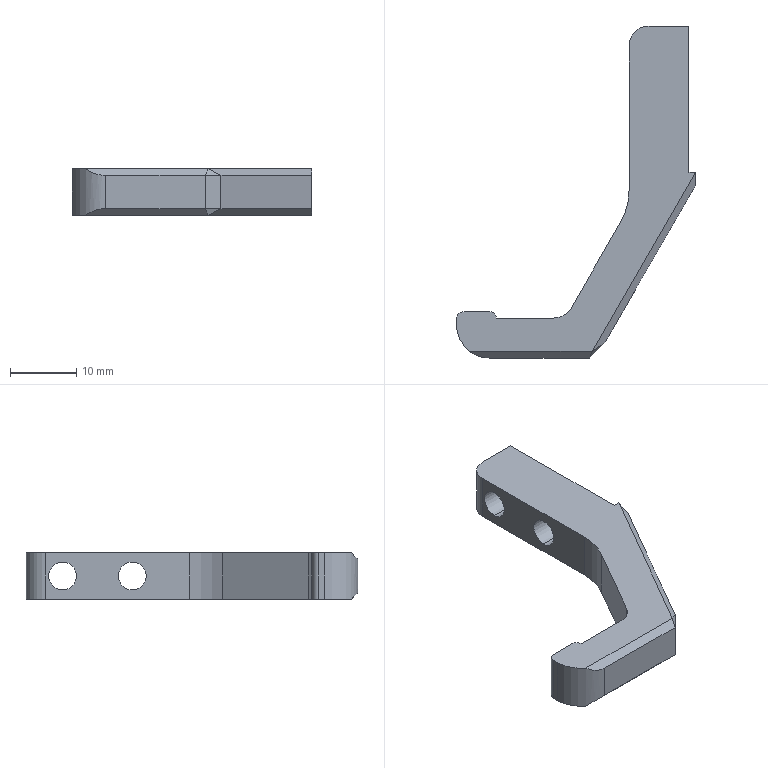Part | NX | features BREP 1 | 1 solid | 30 faces | box 36 x 49.981 x 7 mm | volume 3323 mm3 | plane 20 | cylinder 10 | commonest cylinder face diameters 4.2 x4 2 x2 6 x2 10 x1 20 x1
STEP:
#1=CARTESIAN_POINT('',(733.282,0.5081,5.6));
#2=VERTEX_POINT('',#1);
#3=CARTESIAN_POINT('',(733.282,0.5081,1.4));
#4=VERTEX_POINT('',#3);
#5=CARTESIAN_POINT('',(733.282,0.5081,3.5));
#6=DIRECTION('',(1.,0.,0.));
#7=DIRECTION('',(0.,1.,0.));
#8=AXIS2_PLACEMENT_3D('',#5,#6,#7);
#9=CIRCLE('',#8,2.1);
#10=EDGE_CURVE('',#2,#4,#9,.T.);
#11=ORIENTED_EDGE('',*,*,#10,.F.);
#12=CARTESIAN_POINT('',(742.282,0.5081,5.6));
#13=VERTEX_POINT('',#12);
#14=CARTESIAN_POINT('',(742.282,0.5081,5.6));
#15=DIRECTION('',(1.,0.,0.));
#16=VECTOR('',#15,1000.);
#17=LINE('',#14,#16);
#18=EDGE_CURVE('',#2,#13,#17,.T.);
#19=ORIENTED_EDGE('',*,*,#18,.T.);
#20=CARTESIAN_POINT('',(742.282,0.5081,1.4));
#21=VERTEX_POINT('',#20);
#22=CARTESIAN_POINT('',(742.282,0.5081,3.5));
#23=DIRECTION('',(1.,0.,0.));
#24=DIRECTION('',(0.,0.,-1.));
#25=AXIS2_PLACEMENT_3D('',#22,#23,#24);
#26=CIRCLE('',#25,2.1);
#27=EDGE_CURVE('',#13,#21,#26,.T.);
#28=ORIENTED_EDGE('',*,*,#27,.T.);
#29=CARTESIAN_POINT('',(742.282,0.5081,1.4));
#30=DIRECTION('',(1.,0.,0.));
#31=VECTOR('',#30,1000.);
#32=LINE('',#29,#31);
#33=EDGE_CURVE('',#4,#21,#32,.T.);
#34=ORIENTED_EDGE('',*,*,#33,.F.);
#35=EDGE_LOOP('',(#11,#19,#28,#34));
#36=FACE_BOUND('',#35,.T.);
#37=CARTESIAN_POINT('',(742.282,0.5081,3.5));
#38=DIRECTION('',(1.,0.,0.));
#39=DIRECTION('',(0.,0.,-1.));
#40=AXIS2_PLACEMENT_3D('',#37,#38,#39);
#41=CYLINDRICAL_SURFACE('',#40,2.1);
#42=ADVANCED_FACE('',(#36),#41,.F.);
#43=CARTESIAN_POINT('',(733.282,11.008,5.6));
#44=VERTEX_POINT('',#43);
#45=CARTESIAN_POINT('',(733.282,11.008,1.4));
#46=VERTEX_POINT('',#45);
#47=CARTESIAN_POINT('',(733.282,11.008,3.5));
#48=DIRECTION('',(1.,0.,0.));
#49=DIRECTION('',(0.,1.,0.));
#50=AXIS2_PLACEMENT_3D('',#47,#48,#49);
#51=CIRCLE('',#50,2.1);
#52=EDGE_CURVE('',#44,#46,#51,.T.);
#53=ORIENTED_EDGE('',*,*,#52,.F.);
#54=CARTESIAN_POINT('',(742.282,11.008,5.6));
#55=VERTEX_POINT('',#54);
#56=CARTESIAN_POINT('',(742.282,11.008,5.6));
#57=DIRECTION('',(1.,0.,0.));
#58=VECTOR('',#57,1000.);
#59=LINE('',#56,#58);
#60=EDGE_CURVE('',#44,#55,#59,.T.);
#61=ORIENTED_EDGE('',*,*,#60,.T.);
#62=CARTESIAN_POINT('',(742.282,11.008,1.4));
#63=VERTEX_POINT('',#62);
#64=CARTESIAN_POINT('',(742.282,11.008,3.5));
#65=DIRECTION('',(1.,0.,0.));
#66=DIRECTION('',(0.,0.,-1.));
#67=AXIS2_PLACEMENT_3D('',#64,#65,#66);
#68=CIRCLE('',#67,2.1);
#69=EDGE_CURVE('',#55,#63,#68,.T.);
#70=ORIENTED_EDGE('',*,*,#69,.T.);
#71=CARTESIAN_POINT('',(742.282,11.008,1.4));
#72=DIRECTION('',(1.,0.,0.));
#73=VECTOR('',#72,1000.);
#74=LINE('',#71,#73);
#75=EDGE_CURVE('',#46,#63,#74,.T.);
#76=ORIENTED_EDGE('',*,*,#75,.F.);
#77=EDGE_LOOP('',(#53,#61,#70,#76));
#78=FACE_BOUND('',#77,.T.);
#79=CARTESIAN_POINT('',(742.282,11.008,3.5));
#80=DIRECTION('',(1.,0.,0.));
#81=DIRECTION('',(0.,0.,-1.));
#82=AXIS2_PLACEMENT_3D('',#79,#80,#81);
#83=CYLINDRICAL_SURFACE('',#82,2.1);
#84=ADVANCED_FACE('',(#78),#83,.F.);
#85=CARTESIAN_POINT('',(707.282,-27.556,7.));
#86=VERTEX_POINT('',#85);
#87=CARTESIAN_POINT('',(707.282,-28.473,7.));
#88=VERTEX_POINT('',#87);
#89=CARTESIAN_POINT('',(707.282,-26.473,7.));
#90=DIRECTION('',(0.,-1.,0.));
#91=VECTOR('',#90,1000.);
#92=LINE('',#89,#91);
#93=EDGE_CURVE('',#86,#88,#92,.T.);
#94=ORIENTED_EDGE('',*,*,#93,.F.);
#95=CARTESIAN_POINT('',(707.282,-27.556,0.));
#96=VERTEX_POINT('',#95);
#97=CARTESIAN_POINT('',(707.282,-27.556,0.));
#98=DIRECTION('',(0.,0.,-1.));
#99=VECTOR('',#98,1000.);
#100=LINE('',#97,#99);
#101=EDGE_CURVE('',#86,#96,#100,.T.);
#102=ORIENTED_EDGE('',*,*,#101,.T.);
#103=CARTESIAN_POINT('',(707.282,-28.473,0.));
#104=VERTEX_POINT('',#103);
#105=CARTESIAN_POINT('',(707.282,-26.473,0.));
#106=DIRECTION('',(0.,-1.,0.));
#107=VECTOR('',#106,1000.);
#108=LINE('',#105,#107);
#109=EDGE_CURVE('',#96,#104,#108,.T.);
#110=ORIENTED_EDGE('',*,*,#109,.T.);
#111=CARTESIAN_POINT('',(707.282,-28.473,7.));
#112=DIRECTION('',(0.,0.,1.));
#113=VECTOR('',#112,1000.);
#114=LINE('',#111,#113);
#115=EDGE_CURVE('',#104,#88,#114,.T.);
#116=ORIENTED_EDGE('',*,*,#115,.T.);
#117=EDGE_LOOP('',(#94,#102,#110,#116));
#118=FACE_BOUND('',#117,.T.);
#119=CARTESIAN_POINT('',(707.282,-26.473,7.));
#120=DIRECTION('',(1.,0.,0.));
#121=DIRECTION('',(0.,1.,0.));
#122=AXIS2_PLACEMENT_3D('',#119,#120,#121);
#123=PLANE('',#122);
#124=ADVANCED_FACE('',(#118),#123,.F.);
#125=CARTESIAN_POINT('',(712.265,-26.49,7.));
#126=VERTEX_POINT('',#125);
#127=CARTESIAN_POINT('',(708.265,-26.556,7.));
#128=VERTEX_POINT('',#127);
#129=CARTESIAN_POINT('',(707.167,-26.575,7.));
#130=DIRECTION('',(-0.9999,-0.01666,0.));
#131=VECTOR('',#130,1000.);
#132=LINE('',#129,#131);
#133=EDGE_CURVE('',#126,#128,#132,.T.);
#134=ORIENTED_EDGE('',*,*,#133,.T.);
#135=CARTESIAN_POINT('',(708.282,-27.556,7.));
#136=DIRECTION('',(0.,0.,1.));
#137=DIRECTION('',(1.,0.,0.));
#138=AXIS2_PLACEMENT_3D('',#135,#136,#137);
#139=CIRCLE('',#138,1.);
#140=EDGE_CURVE('',#128,#86,#139,.T.);
#141=ORIENTED_EDGE('',*,*,#140,.T.);
#142=ORIENTED_EDGE('',*,*,#93,.T.);
#143=CARTESIAN_POINT('',(709.282,-32.473,7.));
#144=VERTEX_POINT('',#143);
#145=CARTESIAN_POINT('',(712.282,-28.473,7.));
#146=DIRECTION('',(0.,0.,1.));
#147=DIRECTION('',(1.,0.,0.));
#148=AXIS2_PLACEMENT_3D('',#145,#146,#147);
#149=CIRCLE('',#148,5.);
#150=EDGE_CURVE('',#88,#144,#149,.T.);
#151=ORIENTED_EDGE('',*,*,#150,.T.);
#152=CARTESIAN_POINT('',(727.704,-32.473,7.));
#153=VERTEX_POINT('',#152);
#154=CARTESIAN_POINT('',(728.282,-32.473,7.));
#155=DIRECTION('',(1.,0.,0.));
#156=VECTOR('',#155,1000.);
#157=LINE('',#154,#156);
#158=EDGE_CURVE('',#144,#153,#157,.T.);
#159=ORIENTED_EDGE('',*,*,#158,.T.);
#160=CARTESIAN_POINT('',(743.282,-5.492,7.));
#161=VERTEX_POINT('',#160);
#162=CARTESIAN_POINT('',(742.416,-6.992,7.));
#163=DIRECTION('',(0.5,0.866,0.));
#164=VECTOR('',#163,1000.);
#165=LINE('',#162,#164);
#166=EDGE_CURVE('',#153,#161,#165,.T.);
#167=ORIENTED_EDGE('',*,*,#166,.T.);
#168=CARTESIAN_POINT('',(742.282,-5.492,7.));
#169=VERTEX_POINT('',#168);
#170=CARTESIAN_POINT('',(743.282,-5.492,7.));
#171=DIRECTION('',(1.,0.,0.));
#172=VECTOR('',#171,1000.);
#173=LINE('',#170,#172);
#174=EDGE_CURVE('',#169,#161,#173,.T.);
#175=ORIENTED_EDGE('',*,*,#174,.F.);
#176=CARTESIAN_POINT('',(742.282,16.508,7.));
#177=VERTEX_POINT('',#176);
#178=CARTESIAN_POINT('',(742.282,-5.492,7.));
#179=DIRECTION('',(0.,-1.,0.));
#180=VECTOR('',#179,1000.);
#181=LINE('',#178,#180);
#182=EDGE_CURVE('',#177,#169,#181,.T.);
#183=ORIENTED_EDGE('',*,*,#182,.F.);
#184=CARTESIAN_POINT('',(736.282,16.508,7.));
#185=VERTEX_POINT('',#184);
#186=CARTESIAN_POINT('',(743.282,16.508,7.));
#187=DIRECTION('',(-1.,0.,0.));
#188=VECTOR('',#187,1000.);
#189=LINE('',#186,#188);
#190=EDGE_CURVE('',#177,#185,#189,.T.);
#191=ORIENTED_EDGE('',*,*,#190,.T.);
#192=CARTESIAN_POINT('',(733.282,13.508,7.));
#193=VERTEX_POINT('',#192);
#194=CARTESIAN_POINT('',(736.282,13.508,7.));
#195=DIRECTION('',(0.,0.,1.));
#196=DIRECTION('',(1.,0.,0.));
#197=AXIS2_PLACEMENT_3D('',#194,#195,#196);
#198=CIRCLE('',#197,3.);
#199=EDGE_CURVE('',#185,#193,#198,.T.);
#200=ORIENTED_EDGE('',*,*,#199,.T.);
#201=CARTESIAN_POINT('',(733.282,-8.133,7.));
#202=VERTEX_POINT('',#201);
#203=CARTESIAN_POINT('',(733.282,-10.812,7.));
#204=DIRECTION('',(0.,-1.,0.));
#205=VECTOR('',#204,1000.);
#206=LINE('',#203,#205);
#207=EDGE_CURVE('',#193,#202,#206,.T.);
#208=ORIENTED_EDGE('',*,*,#207,.T.);
#209=CARTESIAN_POINT('',(731.942,-13.133,7.));
#210=VERTEX_POINT('',#209);
#211=CARTESIAN_POINT('',(723.282,-8.133,7.));
#212=DIRECTION('',(0.,0.,-1.));
#213=DIRECTION('',(1.,0.,0.));
#214=AXIS2_PLACEMENT_3D('',#211,#212,#213);
#215=CIRCLE('',#214,10.);
#216=EDGE_CURVE('',#202,#210,#215,.T.);
#217=ORIENTED_EDGE('',*,*,#216,.T.);
#218=CARTESIAN_POINT('',(724.529,-25.973,7.));
#219=VERTEX_POINT('',#218);
#220=CARTESIAN_POINT('',(724.24,-26.473,7.));
#221=DIRECTION('',(-0.5,-0.866,0.));
#222=VECTOR('',#221,1000.);
#223=LINE('',#220,#222);
#224=EDGE_CURVE('',#210,#219,#223,.T.);
#225=ORIENTED_EDGE('',*,*,#224,.T.);
#226=CARTESIAN_POINT('',(721.931,-27.473,7.));
#227=VERTEX_POINT('',#226);
#228=CARTESIAN_POINT('',(721.931,-24.473,7.));
#229=DIRECTION('',(0.,0.,-1.));
#230=DIRECTION('',(1.,0.,0.));
#231=AXIS2_PLACEMENT_3D('',#228,#229,#230);
#232=CIRCLE('',#231,3.);
#233=EDGE_CURVE('',#219,#227,#232,.T.);
#234=ORIENTED_EDGE('',*,*,#233,.T.);
#235=CARTESIAN_POINT('',(713.282,-27.473,7.));
#236=VERTEX_POINT('',#235);
#237=CARTESIAN_POINT('',(723.663,-27.473,7.));
#238=DIRECTION('',(1.,0.,0.));
#239=VECTOR('',#238,1000.);
#240=LINE('',#237,#239);
#241=EDGE_CURVE('',#236,#227,#240,.T.);
#242=ORIENTED_EDGE('',*,*,#241,.F.);
#243=CARTESIAN_POINT('',(712.282,-27.489,7.));
#244=DIRECTION('',(0.,0.,1.));
#245=DIRECTION('',(1.,0.,0.));
#246=AXIS2_PLACEMENT_3D('',#243,#244,#245);
#247=CIRCLE('',#246,1.);
#248=EDGE_CURVE('',#236,#126,#247,.T.);
#249=ORIENTED_EDGE('',*,*,#248,.T.);
#250=EDGE_LOOP('',(#134,#141,#142,#151,#159,#167,#175,#183,#191,#200,#208,#217,#225,#234,#242,#249));
#251=FACE_BOUND('',#250,.T.);
#252=CARTESIAN_POINT('',(707.282,-33.473,7.));
#253=DIRECTION('',(0.,0.,1.));
#254=DIRECTION('',(1.,0.,0.));
#255=AXIS2_PLACEMENT_3D('',#252,#253,#254);
#256=PLANE('',#255);
#257=ADVANCED_FACE('',(#251),#256,.T.);
#258=ORIENTED_EDGE('',*,*,#109,.F.);
#259=CARTESIAN_POINT('',(708.265,-26.556,0.));
#260=VERTEX_POINT('',#259);
#261=CARTESIAN_POINT('',(708.282,-27.556,0.));
#262=DIRECTION('',(0.,0.,-1.));
#263=DIRECTION('',(1.,0.,0.));
#264=AXIS2_PLACEMENT_3D('',#261,#262,#263);
#265=CIRCLE('',#264,1.);
#266=EDGE_CURVE('',#96,#260,#265,.T.);
#267=ORIENTED_EDGE('',*,*,#266,.T.);
#268=CARTESIAN_POINT('',(712.265,-26.49,0.));
#269=VERTEX_POINT('',#268);
#270=CARTESIAN_POINT('',(707.167,-26.575,0.));
#271=DIRECTION('',(-0.9999,-0.01666,0.));
#272=VECTOR('',#271,1000.);
#273=LINE('',#270,#272);
#274=EDGE_CURVE('',#269,#260,#273,.T.);
#275=ORIENTED_EDGE('',*,*,#274,.F.);
#276=CARTESIAN_POINT('',(713.282,-27.473,0.));
#277=VERTEX_POINT('',#276);
#278=CARTESIAN_POINT('',(712.282,-27.489,0.));
#279=DIRECTION('',(0.,0.,-1.));
#280=DIRECTION('',(1.,0.,0.));
#281=AXIS2_PLACEMENT_3D('',#278,#279,#280);
#282=CIRCLE('',#281,1.);
#283=EDGE_CURVE('',#269,#277,#282,.T.);
#284=ORIENTED_EDGE('',*,*,#283,.T.);
#285=CARTESIAN_POINT('',(721.931,-27.473,0.));
#286=VERTEX_POINT('',#285);
#287=CARTESIAN_POINT('',(723.663,-27.473,0.));
#288=DIRECTION('',(1.,0.,0.));
#289=VECTOR('',#288,1000.);
#290=LINE('',#287,#289);
#291=EDGE_CURVE('',#277,#286,#290,.T.);
#292=ORIENTED_EDGE('',*,*,#291,.T.);
#293=CARTESIAN_POINT('',(724.529,-25.973,0.));
#294=VERTEX_POINT('',#293);
#295=CARTESIAN_POINT('',(721.931,-24.473,0.));
#296=DIRECTION('',(0.,0.,1.));
#297=DIRECTION('',(1.,0.,0.));
#298=AXIS2_PLACEMENT_3D('',#295,#296,#297);
#299=CIRCLE('',#298,3.);
#300=EDGE_CURVE('',#286,#294,#299,.T.);
#301=ORIENTED_EDGE('',*,*,#300,.T.);
#302=CARTESIAN_POINT('',(731.942,-13.133,0.));
#303=VERTEX_POINT('',#302);
#304=CARTESIAN_POINT('',(724.24,-26.473,0.));
#305=DIRECTION('',(-0.5,-0.866,0.));
#306=VECTOR('',#305,1000.);
#307=LINE('',#304,#306);
#308=EDGE_CURVE('',#303,#294,#307,.T.);
#309=ORIENTED_EDGE('',*,*,#308,.F.);
#310=CARTESIAN_POINT('',(733.282,-8.133,0.));
#311=VERTEX_POINT('',#310);
#312=CARTESIAN_POINT('',(723.282,-8.133,0.));
#313=DIRECTION('',(0.,0.,1.));
#314=DIRECTION('',(1.,0.,0.));
#315=AXIS2_PLACEMENT_3D('',#312,#313,#314);
#316=CIRCLE('',#315,10.);
#317=EDGE_CURVE('',#303,#311,#316,.T.);
#318=ORIENTED_EDGE('',*,*,#317,.T.);
#319=CARTESIAN_POINT('',(733.282,13.508,0.));
#320=VERTEX_POINT('',#319);
#321=CARTESIAN_POINT('',(733.282,-10.812,0.));
#322=DIRECTION('',(0.,-1.,0.));
#323=VECTOR('',#322,1000.);
#324=LINE('',#321,#323);
#325=EDGE_CURVE('',#320,#311,#324,.T.);
#326=ORIENTED_EDGE('',*,*,#325,.F.);
#327=CARTESIAN_POINT('',(736.282,16.508,0.));
#328=VERTEX_POINT('',#327);
#329=CARTESIAN_POINT('',(736.282,13.508,0.));
#330=DIRECTION('',(0.,0.,-1.));
#331=DIRECTION('',(1.,0.,0.));
#332=AXIS2_PLACEMENT_3D('',#329,#330,#331);
#333=CIRCLE('',#332,3.);
#334=EDGE_CURVE('',#320,#328,#333,.T.);
#335=ORIENTED_EDGE('',*,*,#334,.T.);
#336=CARTESIAN_POINT('',(742.282,16.508,0.));
#337=VERTEX_POINT('',#336);
#338=CARTESIAN_POINT('',(743.282,16.508,0.));
#339=DIRECTION('',(-1.,0.,0.));
#340=VECTOR('',#339,1000.);
#341=LINE('',#338,#340);
#342=EDGE_CURVE('',#337,#328,#341,.T.);
#343=ORIENTED_EDGE('',*,*,#342,.F.);
#344=CARTESIAN_POINT('',(742.282,-5.492,0.));
#345=VERTEX_POINT('',#344);
#346=CARTESIAN_POINT('',(742.282,-5.492,0.));
#347=DIRECTION('',(0.,-1.,0.));
#348=VECTOR('',#347,1000.);
#349=LINE('',#346,#348);
#350=EDGE_CURVE('',#337,#345,#349,.T.);
#351=ORIENTED_EDGE('',*,*,#350,.T.);
#352=CARTESIAN_POINT('',(743.282,-5.492,0.));
#353=VERTEX_POINT('',#352);
#354=CARTESIAN_POINT('',(743.282,-5.492,0.));
#355=DIRECTION('',(1.,0.,0.));
#356=VECTOR('',#355,1000.);
#357=LINE('',#354,#356);
#358=EDGE_CURVE('',#345,#353,#357,.T.);
#359=ORIENTED_EDGE('',*,*,#358,.T.);
#360=CARTESIAN_POINT('',(727.704,-32.473,0.));
#361=VERTEX_POINT('',#360);
#362=CARTESIAN_POINT('',(722.166,-42.066,0.));
#363=DIRECTION('',(-0.5,-0.866,0.));
#364=VECTOR('',#363,1000.);
#365=LINE('',#362,#364);
#366=EDGE_CURVE('',#353,#361,#365,.T.);
#367=ORIENTED_EDGE('',*,*,#366,.T.);
#368=CARTESIAN_POINT('',(709.282,-32.473,0.));
#369=VERTEX_POINT('',#368);
#370=CARTESIAN_POINT('',(707.282,-32.473,0.));
#371=DIRECTION('',(-1.,0.,0.));
#372=VECTOR('',#371,1000.);
#373=LINE('',#370,#372);
#374=EDGE_CURVE('',#361,#369,#373,.T.);
#375=ORIENTED_EDGE('',*,*,#374,.T.);
#376=CARTESIAN_POINT('',(712.282,-28.473,0.));
#377=DIRECTION('',(0.,0.,-1.));
#378=DIRECTION('',(1.,0.,0.));
#379=AXIS2_PLACEMENT_3D('',#376,#377,#378);
#380=CIRCLE('',#379,5.);
#381=EDGE_CURVE('',#369,#104,#380,.T.);
#382=ORIENTED_EDGE('',*,*,#381,.T.);
#383=EDGE_LOOP('',(#258,#267,#275,#284,#292,#301,#309,#318,#326,#335,#343,#351,#359,#367,#375,#382));
#384=FACE_BOUND('',#383,.T.);
#385=CARTESIAN_POINT('',(707.282,-33.473,0.));
#386=DIRECTION('',(0.,0.,1.));
#387=DIRECTION('',(1.,0.,0.));
#388=AXIS2_PLACEMENT_3D('',#385,#386,#387);
#389=PLANE('',#388);
#390=ADVANCED_FACE('',(#384),#389,.F.);
#391=ORIENTED_EDGE('',*,*,#182,.T.);
#392=CARTESIAN_POINT('',(742.282,-5.492,0.));
#393=DIRECTION('',(0.,0.,1.));
#394=VECTOR('',#393,1000.);
#395=LINE('',#392,#394);
#396=EDGE_CURVE('',#345,#169,#395,.T.);
#397=ORIENTED_EDGE('',*,*,#396,.F.);
#398=ORIENTED_EDGE('',*,*,#350,.F.);
#399=CARTESIAN_POINT('',(742.282,16.508,0.));
#400=DIRECTION('',(0.,0.,1.));
#401=VECTOR('',#400,1000.);
#402=LINE('',#399,#401);
#403=EDGE_CURVE('',#337,#177,#402,.T.);
#404=ORIENTED_EDGE('',*,*,#403,.T.);
#405=EDGE_LOOP('',(#391,#397,#398,#404));
#406=FACE_BOUND('',#405,.T.);
#407=CARTESIAN_POINT('',(742.282,0.5081,3.5));
#408=DIRECTION('',(1.,0.,0.));
#409=DIRECTION('',(0.,0.,-1.));
#410=AXIS2_PLACEMENT_3D('',#407,#408,#409);
#411=CIRCLE('',#410,2.1);
#412=EDGE_CURVE('',#21,#13,#411,.T.);
#413=ORIENTED_EDGE('',*,*,#412,.F.);
#414=ORIENTED_EDGE('',*,*,#27,.F.);
#415=EDGE_LOOP('',(#413,#414));
#416=FACE_BOUND('',#415,.T.);
#417=CARTESIAN_POINT('',(742.282,11.008,3.5));
#418=DIRECTION('',(1.,0.,0.));
#419=DIRECTION('',(0.,0.,-1.));
#420=AXIS2_PLACEMENT_3D('',#417,#418,#419);
#421=CIRCLE('',#420,2.1);
#422=EDGE_CURVE('',#63,#55,#421,.T.);
#423=ORIENTED_EDGE('',*,*,#422,.F.);
#424=ORIENTED_EDGE('',*,*,#69,.F.);
#425=EDGE_LOOP('',(#423,#424));
#426=FACE_BOUND('',#425,.T.);
#427=CARTESIAN_POINT('',(742.282,-5.492,0.));
#428=DIRECTION('',(-1.,0.,0.));
#429=DIRECTION('',(0.,0.,1.));
#430=AXIS2_PLACEMENT_3D('',#427,#428,#429);
#431=PLANE('',#430);
#432=ADVANCED_FACE('',(#406,#416,#426),#431,.F.);
#433=CARTESIAN_POINT('',(727.282,-33.473,6.));
#434=VERTEX_POINT('',#433);
#435=CARTESIAN_POINT('',(712.282,-33.473,6.));
#436=VERTEX_POINT('',#435);
#437=CARTESIAN_POINT('',(707.282,-33.473,6.));
#438=DIRECTION('',(-1.,0.,0.));
#439=VECTOR('',#438,1000.);
#440=LINE('',#437,#439);
#441=EDGE_CURVE('',#434,#436,#440,.T.);
#442=ORIENTED_EDGE('',*,*,#441,.T.);
#443=CARTESIAN_POINT('',(712.282,-33.473,1.));
#444=VERTEX_POINT('',#443);
#445=CARTESIAN_POINT('',(712.282,-33.473,7.));
#446=DIRECTION('',(0.,0.,-1.));
#447=VECTOR('',#446,1000.);
#448=LINE('',#445,#447);
#449=EDGE_CURVE('',#436,#444,#448,.T.);
#450=ORIENTED_EDGE('',*,*,#449,.T.);
#451=CARTESIAN_POINT('',(727.282,-33.473,1.));
#452=VERTEX_POINT('',#451);
#453=CARTESIAN_POINT('',(707.282,-33.473,1.));
#454=DIRECTION('',(1.,0.,0.));
#455=VECTOR('',#454,1000.);
#456=LINE('',#453,#455);
#457=EDGE_CURVE('',#444,#452,#456,.T.);
#458=ORIENTED_EDGE('',*,*,#457,.T.);
#459=CARTESIAN_POINT('',(727.282,-33.473,7.));
#460=DIRECTION('',(0.,0.,1.));
#461=VECTOR('',#460,1000.);
#462=LINE('',#459,#461);
#463=EDGE_CURVE('',#452,#434,#462,.T.);
#464=ORIENTED_EDGE('',*,*,#463,.T.);
#465=EDGE_LOOP('',(#442,#450,#458,#464));
#466=FACE_BOUND('',#465,.T.);
#467=CARTESIAN_POINT('',(707.282,-33.473,7.));
#468=DIRECTION('',(0.,1.,0.));
#469=DIRECTION('',(1.,0.,0.));
#470=AXIS2_PLACEMENT_3D('',#467,#468,#469);
#471=PLANE('',#470);
#472=ADVANCED_FACE('',(#466),#471,.F.);
#473=CARTESIAN_POINT('',(729.648,-31.107,6.));
#474=VERTEX_POINT('',#473);
#475=CARTESIAN_POINT('',(729.648,-31.107,1.));
#476=VERTEX_POINT('',#475);
#477=CARTESIAN_POINT('',(729.648,-31.107,7.));
#478=DIRECTION('',(0.,0.,-1.));
#479=VECTOR('',#478,1000.);
#480=LINE('',#477,#479);
#481=EDGE_CURVE('',#474,#476,#480,.T.);
#482=ORIENTED_EDGE('',*,*,#481,.T.);
#483=CARTESIAN_POINT('',(743.282,-7.492,1.));
#484=VERTEX_POINT('',#483);
#485=CARTESIAN_POINT('',(728.282,-33.473,1.));
#486=DIRECTION('',(0.5,0.866,0.));
#487=VECTOR('',#486,1000.);
#488=LINE('',#485,#487);
#489=EDGE_CURVE('',#476,#484,#488,.T.);
#490=ORIENTED_EDGE('',*,*,#489,.T.);
#491=CARTESIAN_POINT('',(743.282,-7.492,6.));
#492=VERTEX_POINT('',#491);
#493=CARTESIAN_POINT('',(743.282,-7.492,7.));
#494=DIRECTION('',(0.,0.,-1.));
#495=VECTOR('',#494,1000.);
#496=LINE('',#493,#495);
#497=EDGE_CURVE('',#492,#484,#496,.T.);
#498=ORIENTED_EDGE('',*,*,#497,.F.);
#499=CARTESIAN_POINT('',(728.282,-33.473,6.));
#500=DIRECTION('',(-0.5,-0.866,0.));
#501=VECTOR('',#500,1000.);
#502=LINE('',#499,#501);
#503=EDGE_CURVE('',#492,#474,#502,.T.);
#504=ORIENTED_EDGE('',*,*,#503,.T.);
#505=EDGE_LOOP('',(#482,#490,#498,#504));
#506=FACE_BOUND('',#505,.T.);
#507=CARTESIAN_POINT('',(728.282,-33.473,7.));
#508=DIRECTION('',(-0.866,0.5,0.));
#509=DIRECTION('',(0.,0.,1.));
#510=AXIS2_PLACEMENT_3D('',#507,#508,#509);
#511=PLANE('',#510);
#512=ADVANCED_FACE('',(#506),#511,.F.);
#513=ORIENTED_EDGE('',*,*,#497,.T.);
#514=CARTESIAN_POINT('',(743.282,-28.277,11.392));
#515=DIRECTION('',(0.,0.8944,-0.4472));
#516=VECTOR('',#515,1000.);
#517=LINE('',#514,#516);
#518=EDGE_CURVE('',#484,#353,#517,.T.);
#519=ORIENTED_EDGE('',*,*,#518,.T.);
#520=CARTESIAN_POINT('',(743.282,-5.492,0.));
#521=DIRECTION('',(0.,0.,1.));
#522=VECTOR('',#521,1000.);
#523=LINE('',#520,#522);
#524=EDGE_CURVE('',#353,#161,#523,.T.);
#525=ORIENTED_EDGE('',*,*,#524,.T.);
#526=CARTESIAN_POINT('',(743.282,-34.751,-7.63));
#527=DIRECTION('',(0.,-0.8944,-0.4472));
#528=VECTOR('',#527,1000.);
#529=LINE('',#526,#528);
#530=EDGE_CURVE('',#161,#492,#529,.T.);
#531=ORIENTED_EDGE('',*,*,#530,.T.);
#532=EDGE_LOOP('',(#513,#519,#525,#531));
#533=FACE_BOUND('',#532,.T.);
#534=CARTESIAN_POINT('',(743.282,-7.492,7.));
#535=DIRECTION('',(-1.,0.,0.));
#536=DIRECTION('',(0.,0.,1.));
#537=AXIS2_PLACEMENT_3D('',#534,#535,#536);
#538=PLANE('',#537);
#539=ADVANCED_FACE('',(#533),#538,.F.);
#540=ORIENTED_EDGE('',*,*,#342,.T.);
#541=CARTESIAN_POINT('',(736.282,16.508,7.));
#542=DIRECTION('',(0.,0.,1.));
#543=VECTOR('',#542,1000.);
#544=LINE('',#541,#543);
#545=EDGE_CURVE('',#328,#185,#544,.T.);
#546=ORIENTED_EDGE('',*,*,#545,.T.);
#547=ORIENTED_EDGE('',*,*,#190,.F.);
#548=ORIENTED_EDGE('',*,*,#403,.F.);
#549=EDGE_LOOP('',(#540,#546,#547,#548));
#550=FACE_BOUND('',#549,.T.);
#551=CARTESIAN_POINT('',(743.282,16.508,7.));
#552=DIRECTION('',(0.,-1.,0.));
#553=DIRECTION('',(-1.,0.,0.));
#554=AXIS2_PLACEMENT_3D('',#551,#552,#553);
#555=PLANE('',#554);
#556=ADVANCED_FACE('',(#550),#555,.F.);
#557=ORIENTED_EDGE('',*,*,#207,.F.);
#558=CARTESIAN_POINT('',(733.282,13.508,7.));
#559=DIRECTION('',(0.,0.,-1.));
#560=VECTOR('',#559,1000.);
#561=LINE('',#558,#560);
#562=EDGE_CURVE('',#193,#320,#561,.T.);
#563=ORIENTED_EDGE('',*,*,#562,.T.);
#564=ORIENTED_EDGE('',*,*,#325,.T.);
#565=CARTESIAN_POINT('',(733.282,-8.133,7.));
#566=DIRECTION('',(0.,0.,1.));
#567=VECTOR('',#566,1000.);
#568=LINE('',#565,#567);
#569=EDGE_CURVE('',#311,#202,#568,.T.);
#570=ORIENTED_EDGE('',*,*,#569,.T.);
#571=EDGE_LOOP('',(#557,#563,#564,#570));
#572=FACE_BOUND('',#571,.T.);
#573=CARTESIAN_POINT('',(733.282,0.5081,3.5));
#574=DIRECTION('',(1.,0.,0.));
#575=DIRECTION('',(0.,1.,0.));
#576=AXIS2_PLACEMENT_3D('',#573,#574,#575);
#577=CIRCLE('',#576,2.1);
#578=EDGE_CURVE('',#4,#2,#577,.T.);
#579=ORIENTED_EDGE('',*,*,#578,.T.);
#580=ORIENTED_EDGE('',*,*,#10,.T.);
#581=EDGE_LOOP('',(#579,#580));
#582=FACE_BOUND('',#581,.T.);
#583=CARTESIAN_POINT('',(733.282,11.008,3.5));
#584=DIRECTION('',(1.,0.,0.));
#585=DIRECTION('',(0.,1.,0.));
#586=AXIS2_PLACEMENT_3D('',#583,#584,#585);
#587=CIRCLE('',#586,2.1);
#588=EDGE_CURVE('',#46,#44,#587,.T.);
#589=ORIENTED_EDGE('',*,*,#588,.T.);
#590=ORIENTED_EDGE('',*,*,#52,.T.);
#591=EDGE_LOOP('',(#589,#590));
#592=FACE_BOUND('',#591,.T.);
#593=CARTESIAN_POINT('',(733.282,-10.812,7.));
#594=DIRECTION('',(1.,0.,0.));
#595=DIRECTION('',(0.,-1.,0.));
#596=AXIS2_PLACEMENT_3D('',#593,#594,#595);
#597=PLANE('',#596);
#598=ADVANCED_FACE('',(#572,#582,#592),#597,.F.);
#599=ORIENTED_EDGE('',*,*,#224,.F.);
#600=CARTESIAN_POINT('',(731.942,-13.133,0.));
#601=DIRECTION('',(0.,0.,-1.));
#602=VECTOR('',#601,1000.);
#603=LINE('',#600,#602);
#604=EDGE_CURVE('',#210,#303,#603,.T.);
#605=ORIENTED_EDGE('',*,*,#604,.T.);
#606=ORIENTED_EDGE('',*,*,#308,.T.);
#607=CARTESIAN_POINT('',(724.529,-25.973,7.));
#608=DIRECTION('',(0.,0.,1.));
#609=VECTOR('',#608,1000.);
#610=LINE('',#607,#609);
#611=EDGE_CURVE('',#294,#219,#610,.T.);
#612=ORIENTED_EDGE('',*,*,#611,.T.);
#613=EDGE_LOOP('',(#599,#605,#606,#612));
#614=FACE_BOUND('',#613,.T.);
#615=CARTESIAN_POINT('',(724.24,-26.473,7.));
#616=DIRECTION('',(0.866,-0.5,0.));
#617=DIRECTION('',(0.,0.,-1.));
#618=AXIS2_PLACEMENT_3D('',#615,#616,#617);
#619=PLANE('',#618);
#620=ADVANCED_FACE('',(#614),#619,.F.);
#621=ORIENTED_EDGE('',*,*,#241,.T.);
#622=CARTESIAN_POINT('',(721.931,-27.473,0.));
#623=DIRECTION('',(0.,0.,-1.));
#624=VECTOR('',#623,1000.);
#625=LINE('',#622,#624);
#626=EDGE_CURVE('',#227,#286,#625,.T.);
#627=ORIENTED_EDGE('',*,*,#626,.T.);
#628=ORIENTED_EDGE('',*,*,#291,.F.);
#629=CARTESIAN_POINT('',(713.282,-27.473,0.));
#630=DIRECTION('',(0.,0.,1.));
#631=VECTOR('',#630,1000.);
#632=LINE('',#629,#631);
#633=EDGE_CURVE('',#277,#236,#632,.T.);
#634=ORIENTED_EDGE('',*,*,#633,.T.);
#635=EDGE_LOOP('',(#621,#627,#628,#634));
#636=FACE_BOUND('',#635,.T.);
#637=CARTESIAN_POINT('',(723.663,-27.473,0.));
#638=DIRECTION('',(0.,-1.,0.));
#639=DIRECTION('',(-1.,0.,0.));
#640=AXIS2_PLACEMENT_3D('',#637,#638,#639);
#641=PLANE('',#640);
#642=ADVANCED_FACE('',(#636),#641,.F.);
#643=ORIENTED_EDGE('',*,*,#300,.F.);
#644=ORIENTED_EDGE('',*,*,#626,.F.);
#645=ORIENTED_EDGE('',*,*,#233,.F.);
#646=ORIENTED_EDGE('',*,*,#611,.F.);
#647=EDGE_LOOP('',(#643,#644,#645,#646));
#648=FACE_BOUND('',#647,.T.);
#649=CARTESIAN_POINT('',(721.931,-24.473,7.));
#650=DIRECTION('',(0.,0.,-1.));
#651=DIRECTION('',(-1.,0.,0.));
#652=AXIS2_PLACEMENT_3D('',#649,#650,#651);
#653=CYLINDRICAL_SURFACE('',#652,3.);
#654=ADVANCED_FACE('',(#648),#653,.F.);
#655=ORIENTED_EDGE('',*,*,#174,.T.);
#656=ORIENTED_EDGE('',*,*,#524,.F.);
#657=ORIENTED_EDGE('',*,*,#358,.F.);
#658=ORIENTED_EDGE('',*,*,#396,.T.);
#659=EDGE_LOOP('',(#655,#656,#657,#658));
#660=FACE_BOUND('',#659,.T.);
#661=CARTESIAN_POINT('',(743.282,-5.492,0.));
#662=DIRECTION('',(0.,-1.,0.));
#663=DIRECTION('',(0.,0.,-1.));
#664=AXIS2_PLACEMENT_3D('',#661,#662,#663);
#665=PLANE('',#664);
#666=ADVANCED_FACE('',(#660),#665,.F.);
#667=ORIENTED_EDGE('',*,*,#216,.F.);
#668=ORIENTED_EDGE('',*,*,#569,.F.);
#669=ORIENTED_EDGE('',*,*,#317,.F.);
#670=ORIENTED_EDGE('',*,*,#604,.F.);
#671=EDGE_LOOP('',(#667,#668,#669,#670));
#672=FACE_BOUND('',#671,.T.);
#673=CARTESIAN_POINT('',(723.282,-8.133,7.));
#674=DIRECTION('',(0.,0.,1.));
#675=DIRECTION('',(1.,0.,0.));
#676=AXIS2_PLACEMENT_3D('',#673,#674,#675);
#677=CYLINDRICAL_SURFACE('',#676,10.);
#678=ADVANCED_FACE('',(#672),#677,.F.);
#679=ORIENTED_EDGE('',*,*,#199,.F.);
#680=ORIENTED_EDGE('',*,*,#545,.F.);
#681=ORIENTED_EDGE('',*,*,#334,.F.);
#682=ORIENTED_EDGE('',*,*,#562,.F.);
#683=EDGE_LOOP('',(#679,#680,#681,#682));
#684=FACE_BOUND('',#683,.T.);
#685=CARTESIAN_POINT('',(736.282,13.508,7.));
#686=DIRECTION('',(0.,0.,-1.));
#687=DIRECTION('',(-1.,0.,0.));
#688=AXIS2_PLACEMENT_3D('',#685,#686,#687);
#689=CYLINDRICAL_SURFACE('',#688,3.);
#690=ADVANCED_FACE('',(#684),#689,.T.);
#691=ORIENTED_EDGE('',*,*,#158,.F.);
#692=CARTESIAN_POINT('',(709.282,-32.473,7.));
#693=CARTESIAN_POINT('',(710.155,-33.128,6.345));
#694=CARTESIAN_POINT('',(711.19,-33.473,6.));
#695=CARTESIAN_POINT('',(712.282,-33.473,6.));
#696=(BOUNDED_CURVE()B_SPLINE_CURVE(3,(#692,#693,#694,#695),.UNSPECIFIED.,.F.,.F.)B_SPLINE_CURVE_WITH_KNOTS((4,4),(5.64,6.283),.UNSPECIFIED.)CURVE()GEOMETRIC_REPRESENTATION_ITEM()RATIONAL_B_SPLINE_CURVE((1.,0.9658,0.9658,1.))REPRESENTATION_ITEM(''));
#697=EDGE_CURVE('',#144,#436,#696,.T.);
#698=ORIENTED_EDGE('',*,*,#697,.T.);
#699=ORIENTED_EDGE('',*,*,#441,.F.);
#700=CARTESIAN_POINT('',(727.282,-33.473,6.));
#701=DIRECTION('',(-0.2863,-0.6775,-0.6775));
#702=VECTOR('',#701,1000.);
#703=LINE('',#700,#702);
#704=EDGE_CURVE('',#153,#434,#703,.T.);
#705=ORIENTED_EDGE('',*,*,#704,.F.);
#706=EDGE_LOOP('',(#691,#698,#699,#705));
#707=FACE_BOUND('',#706,.T.);
#708=CARTESIAN_POINT('',(707.282,-32.473,7.));
#709=DIRECTION('',(0.,-0.7071,0.7071));
#710=DIRECTION('',(-1.,0.,0.));
#711=AXIS2_PLACEMENT_3D('',#708,#709,#710);
#712=PLANE('',#711);
#713=ADVANCED_FACE('',(#707),#712,.T.);
#714=ORIENTED_EDGE('',*,*,#530,.F.);
#715=ORIENTED_EDGE('',*,*,#166,.F.);
#716=CARTESIAN_POINT('',(727.357,-32.717,7.179));
#717=DIRECTION('',(-0.754,-0.53,0.388));
#718=VECTOR('',#717,1000.);
#719=LINE('',#716,#718);
#720=EDGE_CURVE('',#474,#153,#719,.T.);
#721=ORIENTED_EDGE('',*,*,#720,.F.);
#722=ORIENTED_EDGE('',*,*,#503,.F.);
#723=EDGE_LOOP('',(#714,#715,#721,#722));
#724=FACE_BOUND('',#723,.T.);
#725=CARTESIAN_POINT('',(722.166,-42.066,7.));
#726=DIRECTION('',(0.6124,-0.3536,0.7071));
#727=DIRECTION('',(-0.5,-0.866,0.));
#728=AXIS2_PLACEMENT_3D('',#725,#726,#727);
#729=PLANE('',#728);
#730=ADVANCED_FACE('',(#724),#729,.T.);
#731=ORIENTED_EDGE('',*,*,#518,.F.);
#732=ORIENTED_EDGE('',*,*,#489,.F.);
#733=CARTESIAN_POINT('',(729.648,-31.107,1.));
#734=DIRECTION('',(0.754,0.53,0.388));
#735=VECTOR('',#734,1000.);
#736=LINE('',#733,#735);
#737=EDGE_CURVE('',#361,#476,#736,.T.);
#738=ORIENTED_EDGE('',*,*,#737,.F.);
#739=ORIENTED_EDGE('',*,*,#366,.F.);
#740=EDGE_LOOP('',(#731,#732,#738,#739));
#741=FACE_BOUND('',#740,.T.);
#742=CARTESIAN_POINT('',(728.282,-33.473,1.));
#743=DIRECTION('',(-0.6124,0.3536,0.7071));
#744=DIRECTION('',(0.5,0.866,0.));
#745=AXIS2_PLACEMENT_3D('',#742,#743,#744);
#746=PLANE('',#745);
#747=ADVANCED_FACE('',(#741),#746,.F.);
#748=ORIENTED_EDGE('',*,*,#457,.F.);
#749=CARTESIAN_POINT('',(712.282,-33.473,1.));
#750=CARTESIAN_POINT('',(711.19,-33.473,1.));
#751=CARTESIAN_POINT('',(710.155,-33.128,0.6549));
#752=CARTESIAN_POINT('',(709.282,-32.473,0.));
#753=(BOUNDED_CURVE()B_SPLINE_CURVE(3,(#749,#750,#751,#752),.UNSPECIFIED.,.F.,.F.)B_SPLINE_CURVE_WITH_KNOTS((4,4),(3.142,3.785),.UNSPECIFIED.)CURVE()GEOMETRIC_REPRESENTATION_ITEM()RATIONAL_B_SPLINE_CURVE((1.,0.9658,0.9658,1.))REPRESENTATION_ITEM(''));
#754=EDGE_CURVE('',#444,#369,#753,.T.);
#755=ORIENTED_EDGE('',*,*,#754,.T.);
#756=ORIENTED_EDGE('',*,*,#374,.F.);
#757=CARTESIAN_POINT('',(727.935,-31.928,-0.545));
#758=DIRECTION('',(0.2863,0.6775,-0.6775));
#759=VECTOR('',#758,1000.);
#760=LINE('',#757,#759);
#761=EDGE_CURVE('',#452,#361,#760,.T.);
#762=ORIENTED_EDGE('',*,*,#761,.F.);
#763=EDGE_LOOP('',(#748,#755,#756,#762));
#764=FACE_BOUND('',#763,.T.);
#765=CARTESIAN_POINT('',(707.282,-33.473,1.));
#766=DIRECTION('',(0.,0.7071,0.7071));
#767=DIRECTION('',(1.,0.,0.));
#768=AXIS2_PLACEMENT_3D('',#765,#766,#767);
#769=PLANE('',#768);
#770=ADVANCED_FACE('',(#764),#769,.F.);
#771=ORIENTED_EDGE('',*,*,#720,.T.);
#772=ORIENTED_EDGE('',*,*,#704,.T.);
#773=CARTESIAN_POINT('',(727.282,-33.473,6.));
#774=DIRECTION('',(-0.7071,-0.7071,0.));
#775=VECTOR('',#774,1000.);
#776=LINE('',#773,#775);
#777=EDGE_CURVE('',#474,#434,#776,.T.);
#778=ORIENTED_EDGE('',*,*,#777,.F.);
#779=EDGE_LOOP('',(#771,#772,#778));
#780=FACE_BOUND('',#779,.T.);
#781=CARTESIAN_POINT('',(727.282,-33.473,6.));
#782=DIRECTION('',(0.6547,-0.6547,0.378));
#783=DIRECTION('',(0.,-0.5,-0.866));
#784=AXIS2_PLACEMENT_3D('',#781,#782,#783);
#785=PLANE('',#784);
#786=ADVANCED_FACE('',(#780),#785,.T.);
#787=ORIENTED_EDGE('',*,*,#761,.T.);
#788=ORIENTED_EDGE('',*,*,#737,.T.);
#789=CARTESIAN_POINT('',(729.648,-31.107,1.));
#790=DIRECTION('',(0.7071,0.7071,0.));
#791=VECTOR('',#790,1000.);
#792=LINE('',#789,#791);
#793=EDGE_CURVE('',#452,#476,#792,.T.);
#794=ORIENTED_EDGE('',*,*,#793,.F.);
#795=EDGE_LOOP('',(#787,#788,#794));
#796=FACE_BOUND('',#795,.T.);
#797=CARTESIAN_POINT('',(729.648,-31.107,1.));
#798=DIRECTION('',(0.6547,-0.6547,-0.378));
#799=DIRECTION('',(0.,0.5,-0.866));
#800=AXIS2_PLACEMENT_3D('',#797,#798,#799);
#801=PLANE('',#800);
#802=ADVANCED_FACE('',(#796),#801,.T.);
#803=ORIENTED_EDGE('',*,*,#777,.T.);
#804=ORIENTED_EDGE('',*,*,#463,.F.);
#805=ORIENTED_EDGE('',*,*,#793,.T.);
#806=ORIENTED_EDGE('',*,*,#481,.F.);
#807=EDGE_LOOP('',(#803,#804,#805,#806));
#808=FACE_BOUND('',#807,.T.);
#809=CARTESIAN_POINT('',(729.648,-31.107,7.));
#810=DIRECTION('',(-0.7071,0.7071,0.));
#811=DIRECTION('',(0.,0.,1.));
#812=AXIS2_PLACEMENT_3D('',#809,#810,#811);
#813=PLANE('',#812);
#814=ADVANCED_FACE('',(#808),#813,.F.);
#815=ORIENTED_EDGE('',*,*,#60,.F.);
#816=ORIENTED_EDGE('',*,*,#588,.F.);
#817=ORIENTED_EDGE('',*,*,#75,.T.);
#818=ORIENTED_EDGE('',*,*,#422,.T.);
#819=EDGE_LOOP('',(#815,#816,#817,#818));
#820=FACE_BOUND('',#819,.T.);
#821=CARTESIAN_POINT('',(742.282,11.008,3.5));
#822=DIRECTION('',(1.,0.,0.));
#823=DIRECTION('',(0.,0.,-1.));
#824=AXIS2_PLACEMENT_3D('',#821,#822,#823);
#825=CYLINDRICAL_SURFACE('',#824,2.1);
#826=ADVANCED_FACE('',(#820),#825,.F.);
#827=ORIENTED_EDGE('',*,*,#18,.F.);
#828=ORIENTED_EDGE('',*,*,#578,.F.);
#829=ORIENTED_EDGE('',*,*,#33,.T.);
#830=ORIENTED_EDGE('',*,*,#412,.T.);
#831=EDGE_LOOP('',(#827,#828,#829,#830));
#832=FACE_BOUND('',#831,.T.);
#833=CARTESIAN_POINT('',(742.282,0.5081,3.5));
#834=DIRECTION('',(1.,0.,0.));
#835=DIRECTION('',(0.,0.,-1.));
#836=AXIS2_PLACEMENT_3D('',#833,#834,#835);
#837=CYLINDRICAL_SURFACE('',#836,2.1);
#838=ADVANCED_FACE('',(#832),#837,.F.);
#839=ORIENTED_EDGE('',*,*,#150,.F.);
#840=ORIENTED_EDGE('',*,*,#115,.F.);
#841=ORIENTED_EDGE('',*,*,#381,.F.);
#842=ORIENTED_EDGE('',*,*,#754,.F.);
#843=ORIENTED_EDGE('',*,*,#449,.F.);
#844=ORIENTED_EDGE('',*,*,#697,.F.);
#845=EDGE_LOOP('',(#839,#840,#841,#842,#843,#844));
#846=FACE_BOUND('',#845,.T.);
#847=CARTESIAN_POINT('',(712.282,-28.473,7.));
#848=DIRECTION('',(0.,0.,-1.));
#849=DIRECTION('',(-1.,0.,0.));
#850=AXIS2_PLACEMENT_3D('',#847,#848,#849);
#851=CYLINDRICAL_SURFACE('',#850,5.);
#852=ADVANCED_FACE('',(#846),#851,.T.);
#853=ORIENTED_EDGE('',*,*,#274,.T.);
#854=CARTESIAN_POINT('',(708.265,-26.556,7.));
#855=DIRECTION('',(0.,0.,1.));
#856=VECTOR('',#855,1000.);
#857=LINE('',#854,#856);
#858=EDGE_CURVE('',#260,#128,#857,.T.);
#859=ORIENTED_EDGE('',*,*,#858,.T.);
#860=ORIENTED_EDGE('',*,*,#133,.F.);
#861=CARTESIAN_POINT('',(712.265,-26.49,0.));
#862=DIRECTION('',(0.,0.,-1.));
#863=VECTOR('',#862,1000.);
#864=LINE('',#861,#863);
#865=EDGE_CURVE('',#126,#269,#864,.T.);
#866=ORIENTED_EDGE('',*,*,#865,.T.);
#867=EDGE_LOOP('',(#853,#859,#860,#866));
#868=FACE_BOUND('',#867,.T.);
#869=CARTESIAN_POINT('',(713.282,-26.473,-86.241));
#870=DIRECTION('',(-0.01666,0.9999,0.));
#871=DIRECTION('',(0.,0.,1.));
#872=AXIS2_PLACEMENT_3D('',#869,#870,#871);
#873=PLANE('',#872);
#874=ADVANCED_FACE('',(#868),#873,.T.);
#875=ORIENTED_EDGE('',*,*,#266,.F.);
#876=ORIENTED_EDGE('',*,*,#101,.F.);
#877=ORIENTED_EDGE('',*,*,#140,.F.);
#878=ORIENTED_EDGE('',*,*,#858,.F.);
#879=EDGE_LOOP('',(#875,#876,#877,#878));
#880=FACE_BOUND('',#879,.T.);
#881=CARTESIAN_POINT('',(708.282,-27.556,-86.241));
#882=DIRECTION('',(0.,0.,-1.));
#883=DIRECTION('',(-1.,0.,0.));
#884=AXIS2_PLACEMENT_3D('',#881,#882,#883);
#885=CYLINDRICAL_SURFACE('',#884,1.);
#886=ADVANCED_FACE('',(#880),#885,.T.);
#887=ORIENTED_EDGE('',*,*,#283,.F.);
#888=ORIENTED_EDGE('',*,*,#865,.F.);
#889=ORIENTED_EDGE('',*,*,#248,.F.);
#890=ORIENTED_EDGE('',*,*,#633,.F.);
#891=EDGE_LOOP('',(#887,#888,#889,#890));
#892=FACE_BOUND('',#891,.T.);
#893=CARTESIAN_POINT('',(712.282,-27.489,0.));
#894=DIRECTION('',(0.,0.,1.));
#895=DIRECTION('',(1.,0.,0.));
#896=AXIS2_PLACEMENT_3D('',#893,#894,#895);
#897=CYLINDRICAL_SURFACE('',#896,1.);
#898=ADVANCED_FACE('',(#892),#897,.T.);
#899=CLOSED_SHELL('',(#42,#84,#124,#257,#390,#432,#472,#512,#539,#556,#598,#620,#642,#654,#666,#678,#690,#713,#730,#747,#770,#786,#802,#814,#826,#838,#852,#874,#886,#898));
#900=MANIFOLD_SOLID_BREP('',#899);
#901=(LENGTH_UNIT()NAMED_UNIT(*)SI_UNIT(.MILLI.,.METRE.));
#902=UNCERTAINTY_MEASURE_WITH_UNIT(LENGTH_MEASURE(0.00001),#901,'','');
#903=(NAMED_UNIT(*)PLANE_ANGLE_UNIT()SI_UNIT($,.RADIAN.));
#904=(NAMED_UNIT(*)SI_UNIT($,.STERADIAN.)SOLID_ANGLE_UNIT());
#905=(GEOMETRIC_REPRESENTATION_CONTEXT(3)GLOBAL_UNCERTAINTY_ASSIGNED_CONTEXT((#902))GLOBAL_UNIT_ASSIGNED_CONTEXT((#901,#903,#904))REPRESENTATION_CONTEXT('',''));
#906=ADVANCED_BREP_SHAPE_REPRESENTATION('',(#900),#905);